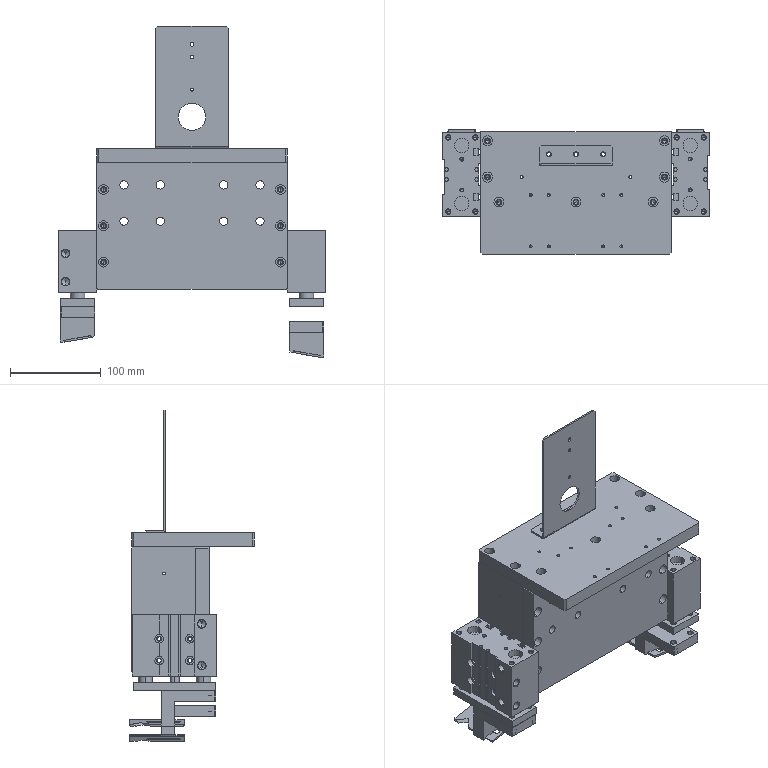Part | SolidWorks | 13 solids | 851 faces | box 294 x 137.5 x 365.515 mm | volume 1735490 mm3 | cylinder 382 | plane 287 | cone 182 | commonest cylinder face diameters 4.917 x48 4 x40 6.6 x34 11 x34 5 x31 3.3 x26